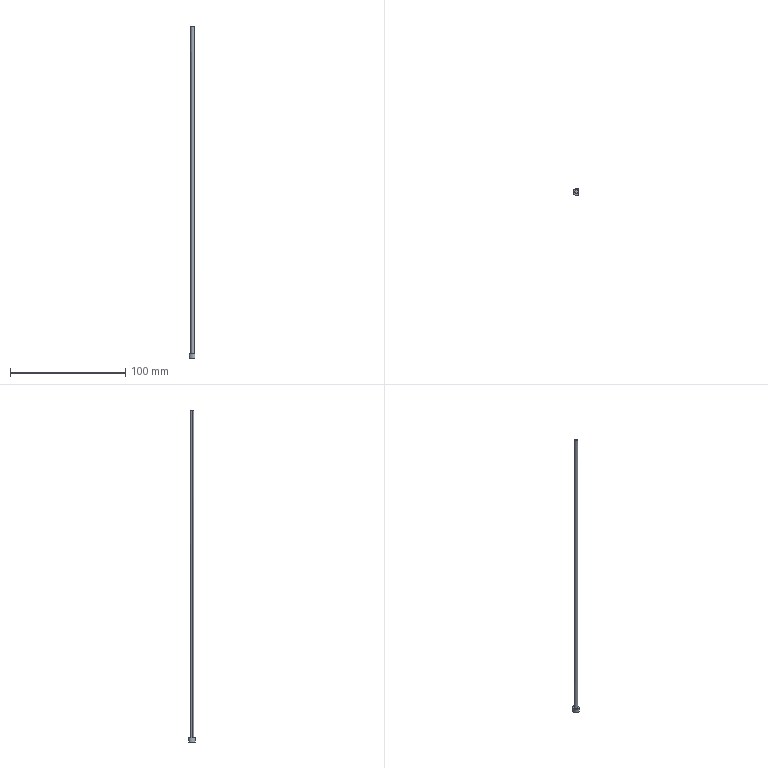Part | Creo | 1 solid | 7 faces | box 5 x 6 x 288.653 mm | volume 2111 mm3 | plane 4 | cylinder 3 | commonest cylinder face diameters 3 x2 6 x1
STEP:
#1=CARTESIAN_POINT('',(82.5,73.5,-292.));
#2=VERTEX_POINT('',#1);
#3=CARTESIAN_POINT('',(79.5,73.5,-292.));
#4=VERTEX_POINT('',#3);
#5=CARTESIAN_POINT('',(81.,73.5,-292.));
#6=DIRECTION('',(0.,0.,-1.));
#7=DIRECTION('',(1.,0.,0.));
#8=AXIS2_PLACEMENT_3D('',#5,#6,#7);
#9=CIRCLE('',#8,1.5);
#10=EDGE_CURVE('',#2,#4,#9,.T.);
#11=ORIENTED_EDGE('',*,*,#10,.T.);
#12=CARTESIAN_POINT('',(79.5,73.5,-7.347));
#13=VERTEX_POINT('',#12);
#14=CARTESIAN_POINT('',(79.5,73.5,-7.347));
#15=DIRECTION('',(0.,0.000000001,-1.));
#16=VECTOR('',#15,284.653);
#17=LINE('',#14,#16);
#18=EDGE_CURVE('',#13,#4,#17,.T.);
#19=ORIENTED_EDGE('',*,*,#18,.F.);
#20=CARTESIAN_POINT('',(82.5,73.5,-7.504));
#21=VERTEX_POINT('',#20);
#22=CARTESIAN_POINT('',(82.5,73.5,-7.504));
#23=CARTESIAN_POINT('',(82.5,73.146,-7.504));
#24=CARTESIAN_POINT('',(82.277,72.523,-7.492));
#25=CARTESIAN_POINT('',(81.554,72.064,-7.454));
#26=CARTESIAN_POINT('',(81.,71.968,-7.425));
#27=CARTESIAN_POINT('',(80.446,72.064,-7.396));
#28=CARTESIAN_POINT('',(79.723,72.523,-7.358));
#29=CARTESIAN_POINT('',(79.5,73.146,-7.347));
#30=CARTESIAN_POINT('',(79.5,73.5,-7.347));
#31=B_SPLINE_CURVE_WITH_KNOTS('',3,(#22,#23,#24,#25,#26,#27,#28,#29,#30),.UNSPECIFIED.,.F.,.F.,(4,1,1,1,1,1,4),(0.,0.25,0.375,0.5,0.625,0.75,1.),.UNSPECIFIED.);
#32=EDGE_CURVE('',#21,#13,#31,.T.);
#33=ORIENTED_EDGE('',*,*,#32,.F.);
#34=CARTESIAN_POINT('',(82.5,73.5,-7.504));
#35=DIRECTION('',(0.,-0.000000001,-1.));
#36=VECTOR('',#35,284.496);
#37=LINE('',#34,#36);
#38=EDGE_CURVE('',#21,#2,#37,.T.);
#39=ORIENTED_EDGE('',*,*,#38,.T.);
#40=EDGE_LOOP('',(#11,#19,#33,#39));
#41=FACE_OUTER_BOUND('',#40,.F.);
#42=CARTESIAN_POINT('',(81.,73.5,-5.));
#43=DIRECTION('',(0.,0.,-1.));
#44=DIRECTION('',(1.,0.,0.));
#45=AXIS2_PLACEMENT_3D('',#42,#43,#44);
#46=CYLINDRICAL_SURFACE('',#45,1.5);
#47=ADVANCED_FACE('',(#41),#46,.T.);
#48=CARTESIAN_POINT('',(83.,71.264,-292.));
#49=VERTEX_POINT('',#48);
#50=CARTESIAN_POINT('',(83.,75.736,-292.));
#51=VERTEX_POINT('',#50);
#52=CARTESIAN_POINT('',(83.,71.264,-292.));
#53=DIRECTION('',(0.,1.,0.));
#54=VECTOR('',#53,4.472);
#55=LINE('',#52,#54);
#56=EDGE_CURVE('',#49,#51,#55,.T.);
#57=ORIENTED_EDGE('',*,*,#56,.F.);
#58=CARTESIAN_POINT('',(78.,73.5,-292.));
#59=VERTEX_POINT('',#58);
#60=CARTESIAN_POINT('',(81.,73.5,-292.));
#61=DIRECTION('',(0.,0.,1.));
#62=DIRECTION('',(-1.,0.,0.));
#63=AXIS2_PLACEMENT_3D('',#60,#61,#62);
#64=CIRCLE('',#63,3.);
#65=EDGE_CURVE('',#59,#49,#64,.T.);
#66=ORIENTED_EDGE('',*,*,#65,.F.);
#67=CARTESIAN_POINT('',(81.,73.5,-292.));
#68=DIRECTION('',(0.,0.,1.));
#69=DIRECTION('',(0.6667,0.7454,0.));
#70=AXIS2_PLACEMENT_3D('',#67,#68,#69);
#71=CIRCLE('',#70,3.);
#72=EDGE_CURVE('',#51,#59,#71,.T.);
#73=ORIENTED_EDGE('',*,*,#72,.F.);
#74=EDGE_LOOP('',(#57,#66,#73));
#75=FACE_OUTER_BOUND('',#74,.F.);
#76=ORIENTED_EDGE('',*,*,#10,.F.);
#77=CARTESIAN_POINT('',(81.,73.5,-292.));
#78=DIRECTION('',(0.,0.,-1.));
#79=DIRECTION('',(-1.,0.,0.));
#80=AXIS2_PLACEMENT_3D('',#77,#78,#79);
#81=CIRCLE('',#80,1.5);
#82=EDGE_CURVE('',#4,#2,#81,.T.);
#83=ORIENTED_EDGE('',*,*,#82,.F.);
#84=EDGE_LOOP('',(#76,#83));
#85=FACE_BOUND('',#84,.F.);
#86=CARTESIAN_POINT('',(81.,73.5,-292.));
#87=DIRECTION('',(0.,0.,1.));
#88=DIRECTION('',(-1.,0.,0.));
#89=AXIS2_PLACEMENT_3D('',#86,#87,#88);
#90=PLANE('',#89);
#91=ADVANCED_FACE('',(#75,#85),#90,.T.);
#92=CARTESIAN_POINT('',(83.,71.264,-296.));
#93=VERTEX_POINT('',#92);
#94=CARTESIAN_POINT('',(83.,71.264,-296.));
#95=DIRECTION('',(0.,0.,1.));
#96=VECTOR('',#95,4.);
#97=LINE('',#94,#96);
#98=EDGE_CURVE('',#93,#49,#97,.T.);
#99=ORIENTED_EDGE('',*,*,#98,.T.);
#100=ORIENTED_EDGE('',*,*,#56,.T.);
#101=CARTESIAN_POINT('',(83.,75.736,-296.));
#102=VERTEX_POINT('',#101);
#103=CARTESIAN_POINT('',(83.,75.736,-292.));
#104=DIRECTION('',(0.,0.,-1.));
#105=VECTOR('',#104,4.);
#106=LINE('',#103,#105);
#107=EDGE_CURVE('',#51,#102,#106,.T.);
#108=ORIENTED_EDGE('',*,*,#107,.T.);
#109=CARTESIAN_POINT('',(83.,71.264,-296.));
#110=DIRECTION('',(0.,1.,0.));
#111=VECTOR('',#110,4.472);
#112=LINE('',#109,#111);
#113=EDGE_CURVE('',#93,#102,#112,.T.);
#114=ORIENTED_EDGE('',*,*,#113,.F.);
#115=EDGE_LOOP('',(#99,#100,#108,#114));
#116=FACE_OUTER_BOUND('',#115,.F.);
#117=CARTESIAN_POINT('',(83.,73.5,-296.));
#118=DIRECTION('',(-1.,0.,0.));
#119=DIRECTION('',(0.,0.,1.));
#120=AXIS2_PLACEMENT_3D('',#117,#118,#119);
#121=PLANE('',#120);
#122=ADVANCED_FACE('',(#116),#121,.F.);
#123=ORIENTED_EDGE('',*,*,#98,.F.);
#124=CARTESIAN_POINT('',(78.,73.5,-296.));
#125=VERTEX_POINT('',#124);
#126=CARTESIAN_POINT('',(81.,73.5,-296.));
#127=DIRECTION('',(0.,0.,-1.));
#128=DIRECTION('',(0.6667,-0.7454,0.));
#129=AXIS2_PLACEMENT_3D('',#126,#127,#128);
#130=CIRCLE('',#129,3.);
#131=EDGE_CURVE('',#93,#125,#130,.T.);
#132=ORIENTED_EDGE('',*,*,#131,.T.);
#133=CARTESIAN_POINT('',(81.,73.5,-296.));
#134=DIRECTION('',(0.,0.,-1.));
#135=DIRECTION('',(-1.,0.,0.));
#136=AXIS2_PLACEMENT_3D('',#133,#134,#135);
#137=CIRCLE('',#136,3.);
#138=EDGE_CURVE('',#125,#102,#137,.T.);
#139=ORIENTED_EDGE('',*,*,#138,.T.);
#140=ORIENTED_EDGE('',*,*,#107,.F.);
#141=ORIENTED_EDGE('',*,*,#72,.T.);
#142=ORIENTED_EDGE('',*,*,#65,.T.);
#143=EDGE_LOOP('',(#123,#132,#139,#140,#141,#142));
#144=FACE_OUTER_BOUND('',#143,.F.);
#145=CARTESIAN_POINT('',(81.,73.5,-296.));
#146=DIRECTION('',(0.,0.,1.));
#147=DIRECTION('',(-1.,0.,0.));
#148=AXIS2_PLACEMENT_3D('',#145,#146,#147);
#149=CYLINDRICAL_SURFACE('',#148,3.);
#150=ADVANCED_FACE('',(#144),#149,.T.);
#151=ORIENTED_EDGE('',*,*,#131,.F.);
#152=ORIENTED_EDGE('',*,*,#113,.T.);
#153=ORIENTED_EDGE('',*,*,#138,.F.);
#154=EDGE_LOOP('',(#151,#152,#153));
#155=FACE_OUTER_BOUND('',#154,.F.);
#156=CARTESIAN_POINT('',(7.7,2.155,-296.));
#157=DIRECTION('',(0.,0.,1.));
#158=DIRECTION('',(0.,-1.,0.));
#159=AXIS2_PLACEMENT_3D('',#156,#157,#158);
#160=PLANE('',#159);
#161=ADVANCED_FACE('',(#155),#160,.F.);
#162=ORIENTED_EDGE('',*,*,#82,.T.);
#163=ORIENTED_EDGE('',*,*,#38,.F.);
#164=CARTESIAN_POINT('',(79.5,73.5,-7.347));
#165=CARTESIAN_POINT('',(79.5,73.854,-7.347));
#166=CARTESIAN_POINT('',(79.723,74.477,-7.358));
#167=CARTESIAN_POINT('',(80.446,74.936,-7.396));
#168=CARTESIAN_POINT('',(81.,75.032,-7.425));
#169=CARTESIAN_POINT('',(81.554,74.936,-7.454));
#170=CARTESIAN_POINT('',(82.277,74.477,-7.492));
#171=CARTESIAN_POINT('',(82.5,73.854,-7.504));
#172=CARTESIAN_POINT('',(82.5,73.5,-7.504));
#173=B_SPLINE_CURVE_WITH_KNOTS('',3,(#164,#165,#166,#167,#168,#169,#170,#171,#172),.UNSPECIFIED.,.F.,.F.,(4,1,1,1,1,1,4),(0.,0.25,0.375,0.5,0.625,0.75,1.),.UNSPECIFIED.);
#174=EDGE_CURVE('',#13,#21,#173,.T.);
#175=ORIENTED_EDGE('',*,*,#174,.F.);
#176=ORIENTED_EDGE('',*,*,#18,.T.);
#177=EDGE_LOOP('',(#162,#163,#175,#176));
#178=FACE_OUTER_BOUND('',#177,.F.);
#179=CARTESIAN_POINT('',(81.,73.5,-5.));
#180=DIRECTION('',(0.,0.,-1.));
#181=DIRECTION('',(1.,0.,0.));
#182=AXIS2_PLACEMENT_3D('',#179,#180,#181);
#183=CYLINDRICAL_SURFACE('',#182,1.5);
#184=ADVANCED_FACE('',(#178),#183,.T.);
#185=ORIENTED_EDGE('',*,*,#174,.T.);
#186=ORIENTED_EDGE('',*,*,#32,.T.);
#187=EDGE_LOOP('',(#185,#186));
#188=FACE_OUTER_BOUND('',#187,.F.);
#189=CARTESIAN_POINT('',(308.361,351.75,-19.338));
#190=DIRECTION('',(0.05232,0.000000032,0.9986));
#191=DIRECTION('',(-0.000000001,1.,-0.000000032));
#192=AXIS2_PLACEMENT_3D('',#189,#190,#191);
#193=PLANE('',#192);
#194=ADVANCED_FACE('',(#188),#193,.T.);
#195=CLOSED_SHELL('',(#47,#91,#122,#150,#161,#184,#194));
#196=MANIFOLD_SOLID_BREP('',#195);
#197=(LENGTH_UNIT()NAMED_UNIT(*)SI_UNIT(.MILLI.,.METRE.));
#198=UNCERTAINTY_MEASURE_WITH_UNIT(LENGTH_MEASURE(0.02887),#197,'','');
#199=(NAMED_UNIT(*)PLANE_ANGLE_UNIT()SI_UNIT($,.RADIAN.));
#200=PLANE_ANGLE_MEASURE_WITH_UNIT(PLANE_ANGLE_MEASURE(0.01745),#199);
#201=(CONVERSION_BASED_UNIT('DEGREE',#200)NAMED_UNIT(*)PLANE_ANGLE_UNIT());
#202=(NAMED_UNIT(*)SI_UNIT($,.STERADIAN.)SOLID_ANGLE_UNIT());
#203=(GEOMETRIC_REPRESENTATION_CONTEXT(3)GLOBAL_UNCERTAINTY_ASSIGNED_CONTEXT((#198))GLOBAL_UNIT_ASSIGNED_CONTEXT((#197,#201,#202))REPRESENTATION_CONTEXT('',''));
#204=ADVANCED_BREP_SHAPE_REPRESENTATION('',(#196),#203);